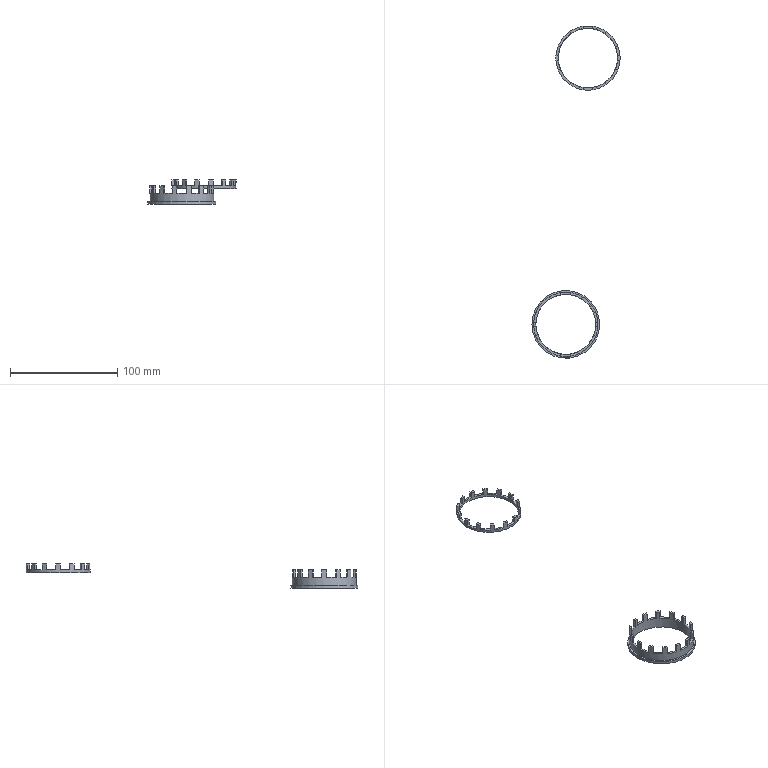Part | 2 solids | 124 faces | box 82.344 x 310.506 x 22.5 mm | volume 6923 mm3 | plane 119 | cylinder 5 | commonest cylinder face diameters 60 x2 55.5 x1 56 x1 63.3 x1